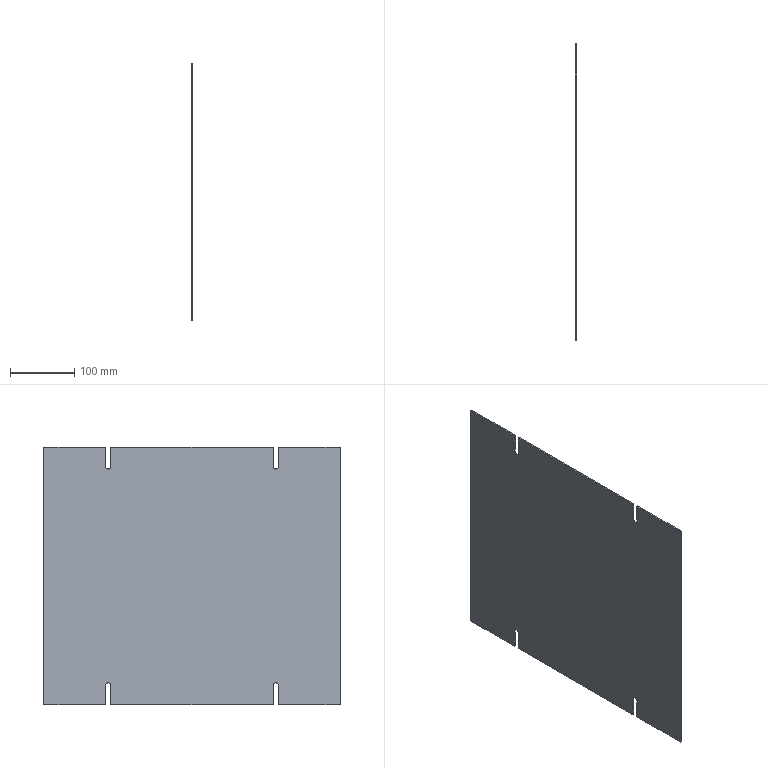Part | STEP file | Pneumatic circuit board | 1 solid | 24 faces | box 2 x 460 x 400 mm | volume 365879 mm3 | plane 18 | cylinder 6 | commonest cylinder face diameters 8 x6
STEP:
#1=CARTESIAN_POINT('',(0.,130.,166.));
#2=VERTEX_POINT('',#1);
#3=CARTESIAN_POINT('',(0.,134.,170.));
#4=VERTEX_POINT('',#3);
#5=CARTESIAN_POINT('',(0.,130.,170.));
#6=DIRECTION('',(1.,0.,0.));
#7=DIRECTION('',(0.,0.,-1.));
#8=AXIS2_PLACEMENT_3D('',#5,#6,#7);
#9=CIRCLE('',#8,4.);
#10=EDGE_CURVE('',#2,#4,#9,.T.);
#11=ORIENTED_EDGE('',*,*,#10,.F.);
#12=CARTESIAN_POINT('',(2.,130.,166.));
#13=VERTEX_POINT('',#12);
#14=CARTESIAN_POINT('',(0.,130.,166.));
#15=DIRECTION('',(1.,0.,0.));
#16=VECTOR('',#15,1000.);
#17=LINE('',#14,#16);
#18=EDGE_CURVE('',#2,#13,#17,.T.);
#19=ORIENTED_EDGE('',*,*,#18,.T.);
#20=CARTESIAN_POINT('',(2.,134.,170.));
#21=VERTEX_POINT('',#20);
#22=CARTESIAN_POINT('',(2.,130.,170.));
#23=DIRECTION('',(1.,0.,0.));
#24=DIRECTION('',(0.,0.,-1.));
#25=AXIS2_PLACEMENT_3D('',#22,#23,#24);
#26=CIRCLE('',#25,4.);
#27=EDGE_CURVE('',#13,#21,#26,.T.);
#28=ORIENTED_EDGE('',*,*,#27,.T.);
#29=CARTESIAN_POINT('',(0.,134.,170.));
#30=DIRECTION('',(-1.,0.,0.));
#31=VECTOR('',#30,1000.);
#32=LINE('',#29,#31);
#33=EDGE_CURVE('',#21,#4,#32,.T.);
#34=ORIENTED_EDGE('',*,*,#33,.T.);
#35=EDGE_LOOP('',(#11,#19,#28,#34));
#36=FACE_OUTER_BOUND('',#35,.T.);
#37=CARTESIAN_POINT('',(0.,130.,170.));
#38=DIRECTION('',(1.,0.,0.));
#39=DIRECTION('',(0.,0.,-1.));
#40=AXIS2_PLACEMENT_3D('',#37,#38,#39);
#41=CYLINDRICAL_SURFACE('',#40,4.);
#42=ADVANCED_FACE('',(#36),#41,.F.);
#43=CARTESIAN_POINT('',(0.,-130.,166.));
#44=VERTEX_POINT('',#43);
#45=CARTESIAN_POINT('',(0.,-126.,170.));
#46=VERTEX_POINT('',#45);
#47=CARTESIAN_POINT('',(0.,-130.,170.));
#48=DIRECTION('',(1.,0.,0.));
#49=DIRECTION('',(0.,0.,-1.));
#50=AXIS2_PLACEMENT_3D('',#47,#48,#49);
#51=CIRCLE('',#50,4.);
#52=EDGE_CURVE('',#44,#46,#51,.T.);
#53=ORIENTED_EDGE('',*,*,#52,.F.);
#54=CARTESIAN_POINT('',(2.,-130.,166.));
#55=VERTEX_POINT('',#54);
#56=CARTESIAN_POINT('',(0.,-130.,166.));
#57=DIRECTION('',(1.,0.,0.));
#58=VECTOR('',#57,1000.);
#59=LINE('',#56,#58);
#60=EDGE_CURVE('',#44,#55,#59,.T.);
#61=ORIENTED_EDGE('',*,*,#60,.T.);
#62=CARTESIAN_POINT('',(2.,-126.,170.));
#63=VERTEX_POINT('',#62);
#64=CARTESIAN_POINT('',(2.,-130.,170.));
#65=DIRECTION('',(1.,0.,0.));
#66=DIRECTION('',(0.,0.,-1.));
#67=AXIS2_PLACEMENT_3D('',#64,#65,#66);
#68=CIRCLE('',#67,4.);
#69=EDGE_CURVE('',#55,#63,#68,.T.);
#70=ORIENTED_EDGE('',*,*,#69,.T.);
#71=CARTESIAN_POINT('',(0.,-126.,170.));
#72=DIRECTION('',(-1.,0.,0.));
#73=VECTOR('',#72,1000.);
#74=LINE('',#71,#73);
#75=EDGE_CURVE('',#63,#46,#74,.T.);
#76=ORIENTED_EDGE('',*,*,#75,.T.);
#77=EDGE_LOOP('',(#53,#61,#70,#76));
#78=FACE_OUTER_BOUND('',#77,.T.);
#79=CARTESIAN_POINT('',(0.,-130.,170.));
#80=DIRECTION('',(1.,0.,0.));
#81=DIRECTION('',(0.,0.,-1.));
#82=AXIS2_PLACEMENT_3D('',#79,#80,#81);
#83=CYLINDRICAL_SURFACE('',#82,4.);
#84=ADVANCED_FACE('',(#78),#83,.F.);
#85=CARTESIAN_POINT('',(2.,134.,-170.));
#86=VERTEX_POINT('',#85);
#87=CARTESIAN_POINT('',(2.,126.,-170.));
#88=VERTEX_POINT('',#87);
#89=CARTESIAN_POINT('',(2.,130.,-170.));
#90=DIRECTION('',(1.,0.,0.));
#91=DIRECTION('',(0.,0.,-1.));
#92=AXIS2_PLACEMENT_3D('',#89,#90,#91);
#93=CIRCLE('',#92,4.);
#94=EDGE_CURVE('',#86,#88,#93,.T.);
#95=ORIENTED_EDGE('',*,*,#94,.F.);
#96=CARTESIAN_POINT('',(2.,134.,-200.));
#97=VERTEX_POINT('',#96);
#98=CARTESIAN_POINT('',(2.,134.,0.));
#99=DIRECTION('',(0.,0.,1.));
#100=VECTOR('',#99,1000.);
#101=LINE('',#98,#100);
#102=EDGE_CURVE('',#97,#86,#101,.T.);
#103=ORIENTED_EDGE('',*,*,#102,.F.);
#104=CARTESIAN_POINT('',(2.,230.,-200.));
#105=VERTEX_POINT('',#104);
#106=CARTESIAN_POINT('',(2.,0.,-200.));
#107=DIRECTION('',(0.,-1.,0.));
#108=VECTOR('',#107,1000.);
#109=LINE('',#106,#108);
#110=EDGE_CURVE('',#105,#97,#109,.T.);
#111=ORIENTED_EDGE('',*,*,#110,.F.);
#112=CARTESIAN_POINT('',(2.,230.,200.));
#113=VERTEX_POINT('',#112);
#114=CARTESIAN_POINT('',(2.,230.,0.));
#115=DIRECTION('',(0.,0.,-1.));
#116=VECTOR('',#115,1000.);
#117=LINE('',#114,#116);
#118=EDGE_CURVE('',#113,#105,#117,.T.);
#119=ORIENTED_EDGE('',*,*,#118,.F.);
#120=CARTESIAN_POINT('',(2.,134.,200.));
#121=VERTEX_POINT('',#120);
#122=CARTESIAN_POINT('',(2.,0.,200.));
#123=DIRECTION('',(0.,1.,0.));
#124=VECTOR('',#123,1000.);
#125=LINE('',#122,#124);
#126=EDGE_CURVE('',#121,#113,#125,.T.);
#127=ORIENTED_EDGE('',*,*,#126,.F.);
#128=CARTESIAN_POINT('',(2.,134.,0.));
#129=DIRECTION('',(0.,0.,1.));
#130=VECTOR('',#129,1000.);
#131=LINE('',#128,#130);
#132=EDGE_CURVE('',#21,#121,#131,.T.);
#133=ORIENTED_EDGE('',*,*,#132,.F.);
#134=ORIENTED_EDGE('',*,*,#27,.F.);
#135=CARTESIAN_POINT('',(2.,126.,170.));
#136=VERTEX_POINT('',#135);
#137=CARTESIAN_POINT('',(2.,130.,170.));
#138=DIRECTION('',(1.,0.,0.));
#139=DIRECTION('',(0.,0.,-1.));
#140=AXIS2_PLACEMENT_3D('',#137,#138,#139);
#141=CIRCLE('',#140,4.);
#142=EDGE_CURVE('',#136,#13,#141,.T.);
#143=ORIENTED_EDGE('',*,*,#142,.F.);
#144=CARTESIAN_POINT('',(2.,126.,200.));
#145=VERTEX_POINT('',#144);
#146=CARTESIAN_POINT('',(2.,126.,0.));
#147=DIRECTION('',(0.,0.,-1.));
#148=VECTOR('',#147,1000.);
#149=LINE('',#146,#148);
#150=EDGE_CURVE('',#145,#136,#149,.T.);
#151=ORIENTED_EDGE('',*,*,#150,.F.);
#152=CARTESIAN_POINT('',(2.,-126.,200.));
#153=VERTEX_POINT('',#152);
#154=CARTESIAN_POINT('',(2.,0.,200.));
#155=DIRECTION('',(0.,1.,0.));
#156=VECTOR('',#155,1000.);
#157=LINE('',#154,#156);
#158=EDGE_CURVE('',#153,#145,#157,.T.);
#159=ORIENTED_EDGE('',*,*,#158,.F.);
#160=CARTESIAN_POINT('',(2.,-126.,0.));
#161=DIRECTION('',(0.,0.,1.));
#162=VECTOR('',#161,1000.);
#163=LINE('',#160,#162);
#164=EDGE_CURVE('',#63,#153,#163,.T.);
#165=ORIENTED_EDGE('',*,*,#164,.F.);
#166=ORIENTED_EDGE('',*,*,#69,.F.);
#167=CARTESIAN_POINT('',(2.,-134.,170.));
#168=VERTEX_POINT('',#167);
#169=CARTESIAN_POINT('',(2.,-130.,170.));
#170=DIRECTION('',(1.,0.,0.));
#171=DIRECTION('',(0.,0.,-1.));
#172=AXIS2_PLACEMENT_3D('',#169,#170,#171);
#173=CIRCLE('',#172,4.);
#174=EDGE_CURVE('',#168,#55,#173,.T.);
#175=ORIENTED_EDGE('',*,*,#174,.F.);
#176=CARTESIAN_POINT('',(2.,-134.,200.));
#177=VERTEX_POINT('',#176);
#178=CARTESIAN_POINT('',(2.,-134.,0.));
#179=DIRECTION('',(0.,0.,-1.));
#180=VECTOR('',#179,1000.);
#181=LINE('',#178,#180);
#182=EDGE_CURVE('',#177,#168,#181,.T.);
#183=ORIENTED_EDGE('',*,*,#182,.F.);
#184=CARTESIAN_POINT('',(2.,-230.,200.));
#185=VERTEX_POINT('',#184);
#186=CARTESIAN_POINT('',(2.,0.,200.));
#187=DIRECTION('',(0.,1.,0.));
#188=VECTOR('',#187,1000.);
#189=LINE('',#186,#188);
#190=EDGE_CURVE('',#185,#177,#189,.T.);
#191=ORIENTED_EDGE('',*,*,#190,.F.);
#192=CARTESIAN_POINT('',(2.,-230.,-200.));
#193=VERTEX_POINT('',#192);
#194=CARTESIAN_POINT('',(2.,-230.,0.));
#195=DIRECTION('',(0.,0.,1.));
#196=VECTOR('',#195,1000.);
#197=LINE('',#194,#196);
#198=EDGE_CURVE('',#193,#185,#197,.T.);
#199=ORIENTED_EDGE('',*,*,#198,.F.);
#200=CARTESIAN_POINT('',(2.,-134.,-200.));
#201=VERTEX_POINT('',#200);
#202=CARTESIAN_POINT('',(2.,0.,-200.));
#203=DIRECTION('',(0.,-1.,0.));
#204=VECTOR('',#203,1000.);
#205=LINE('',#202,#204);
#206=EDGE_CURVE('',#201,#193,#205,.T.);
#207=ORIENTED_EDGE('',*,*,#206,.F.);
#208=CARTESIAN_POINT('',(2.,-134.,-170.));
#209=VERTEX_POINT('',#208);
#210=CARTESIAN_POINT('',(2.,-134.,0.));
#211=DIRECTION('',(0.,0.,-1.));
#212=VECTOR('',#211,1000.);
#213=LINE('',#210,#212);
#214=EDGE_CURVE('',#209,#201,#213,.T.);
#215=ORIENTED_EDGE('',*,*,#214,.F.);
#216=CARTESIAN_POINT('',(2.,-126.,-170.));
#217=VERTEX_POINT('',#216);
#218=CARTESIAN_POINT('',(2.,-130.,-170.));
#219=DIRECTION('',(1.,0.,0.));
#220=DIRECTION('',(0.,0.,-1.));
#221=AXIS2_PLACEMENT_3D('',#218,#219,#220);
#222=CIRCLE('',#221,4.);
#223=EDGE_CURVE('',#217,#209,#222,.T.);
#224=ORIENTED_EDGE('',*,*,#223,.F.);
#225=CARTESIAN_POINT('',(2.,-126.,-200.));
#226=VERTEX_POINT('',#225);
#227=CARTESIAN_POINT('',(2.,-126.,0.));
#228=DIRECTION('',(0.,0.,1.));
#229=VECTOR('',#228,1000.);
#230=LINE('',#227,#229);
#231=EDGE_CURVE('',#226,#217,#230,.T.);
#232=ORIENTED_EDGE('',*,*,#231,.F.);
#233=CARTESIAN_POINT('',(2.,126.,-200.));
#234=VERTEX_POINT('',#233);
#235=CARTESIAN_POINT('',(2.,0.,-200.));
#236=DIRECTION('',(0.,-1.,0.));
#237=VECTOR('',#236,1000.);
#238=LINE('',#235,#237);
#239=EDGE_CURVE('',#234,#226,#238,.T.);
#240=ORIENTED_EDGE('',*,*,#239,.F.);
#241=CARTESIAN_POINT('',(2.,126.,0.));
#242=DIRECTION('',(0.,0.,-1.));
#243=VECTOR('',#242,1000.);
#244=LINE('',#241,#243);
#245=EDGE_CURVE('',#88,#234,#244,.T.);
#246=ORIENTED_EDGE('',*,*,#245,.F.);
#247=EDGE_LOOP('',(#95,#103,#111,#119,#127,#133,#134,#143,#151,#159,#165,#166,#175,#183,#191,#199,#207,#215,#224,#232,#240,#246));
#248=FACE_OUTER_BOUND('',#247,.T.);
#249=CARTESIAN_POINT('',(2.,0.,0.));
#250=DIRECTION('',(-1.,0.,0.));
#251=DIRECTION('',(0.,0.,1.));
#252=AXIS2_PLACEMENT_3D('',#249,#250,#251);
#253=PLANE('',#252);
#254=ADVANCED_FACE('',(#248),#253,.F.);
#255=CARTESIAN_POINT('',(0.,126.,-170.));
#256=VERTEX_POINT('',#255);
#257=CARTESIAN_POINT('',(0.,126.,-170.));
#258=DIRECTION('',(1.,0.,0.));
#259=VECTOR('',#258,1000.);
#260=LINE('',#257,#259);
#261=EDGE_CURVE('',#256,#88,#260,.T.);
#262=ORIENTED_EDGE('',*,*,#261,.T.);
#263=ORIENTED_EDGE('',*,*,#245,.T.);
#264=CARTESIAN_POINT('',(0.,126.,-200.));
#265=VERTEX_POINT('',#264);
#266=CARTESIAN_POINT('',(0.,126.,-200.));
#267=DIRECTION('',(-1.,0.,0.));
#268=VECTOR('',#267,1000.);
#269=LINE('',#266,#268);
#270=EDGE_CURVE('',#234,#265,#269,.T.);
#271=ORIENTED_EDGE('',*,*,#270,.T.);
#272=CARTESIAN_POINT('',(0.,126.,-230.));
#273=DIRECTION('',(0.,0.,1.));
#274=VECTOR('',#273,1000.);
#275=LINE('',#272,#274);
#276=EDGE_CURVE('',#265,#256,#275,.T.);
#277=ORIENTED_EDGE('',*,*,#276,.T.);
#278=EDGE_LOOP('',(#262,#263,#271,#277));
#279=FACE_OUTER_BOUND('',#278,.T.);
#280=CARTESIAN_POINT('',(0.,126.,-230.));
#281=DIRECTION('',(0.,1.,0.));
#282=DIRECTION('',(0.,0.,1.));
#283=AXIS2_PLACEMENT_3D('',#280,#281,#282);
#284=PLANE('',#283);
#285=ADVANCED_FACE('',(#279),#284,.T.);
#286=ORIENTED_EDGE('',*,*,#261,.F.);
#287=CARTESIAN_POINT('',(0.,134.,-170.));
#288=VERTEX_POINT('',#287);
#289=CARTESIAN_POINT('',(0.,130.,-170.));
#290=DIRECTION('',(1.,0.,0.));
#291=DIRECTION('',(0.,0.,-1.));
#292=AXIS2_PLACEMENT_3D('',#289,#290,#291);
#293=CIRCLE('',#292,4.);
#294=EDGE_CURVE('',#288,#256,#293,.T.);
#295=ORIENTED_EDGE('',*,*,#294,.F.);
#296=CARTESIAN_POINT('',(0.,134.,-170.));
#297=DIRECTION('',(-1.,0.,0.));
#298=VECTOR('',#297,1000.);
#299=LINE('',#296,#298);
#300=EDGE_CURVE('',#86,#288,#299,.T.);
#301=ORIENTED_EDGE('',*,*,#300,.F.);
#302=ORIENTED_EDGE('',*,*,#94,.T.);
#303=EDGE_LOOP('',(#286,#295,#301,#302));
#304=FACE_OUTER_BOUND('',#303,.T.);
#305=CARTESIAN_POINT('',(0.,130.,-170.));
#306=DIRECTION('',(1.,0.,0.));
#307=DIRECTION('',(0.,0.,-1.));
#308=AXIS2_PLACEMENT_3D('',#305,#306,#307);
#309=CYLINDRICAL_SURFACE('',#308,4.);
#310=ADVANCED_FACE('',(#304),#309,.F.);
#311=ORIENTED_EDGE('',*,*,#300,.T.);
#312=CARTESIAN_POINT('',(0.,134.,-200.));
#313=VERTEX_POINT('',#312);
#314=CARTESIAN_POINT('',(0.,134.,-230.));
#315=DIRECTION('',(0.,0.,-1.));
#316=VECTOR('',#315,1000.);
#317=LINE('',#314,#316);
#318=EDGE_CURVE('',#288,#313,#317,.T.);
#319=ORIENTED_EDGE('',*,*,#318,.T.);
#320=CARTESIAN_POINT('',(0.,134.,-200.));
#321=DIRECTION('',(1.,0.,0.));
#322=VECTOR('',#321,1000.);
#323=LINE('',#320,#322);
#324=EDGE_CURVE('',#313,#97,#323,.T.);
#325=ORIENTED_EDGE('',*,*,#324,.T.);
#326=ORIENTED_EDGE('',*,*,#102,.T.);
#327=EDGE_LOOP('',(#311,#319,#325,#326));
#328=FACE_OUTER_BOUND('',#327,.T.);
#329=CARTESIAN_POINT('',(0.,134.,-230.));
#330=DIRECTION('',(0.,-1.,0.));
#331=DIRECTION('',(0.,0.,-1.));
#332=AXIS2_PLACEMENT_3D('',#329,#330,#331);
#333=PLANE('',#332);
#334=ADVANCED_FACE('',(#328),#333,.T.);
#335=CARTESIAN_POINT('',(0.,230.,-200.));
#336=VERTEX_POINT('',#335);
#337=CARTESIAN_POINT('',(0.,-230.,-200.));
#338=DIRECTION('',(0.,-1.,0.));
#339=VECTOR('',#338,1000.);
#340=LINE('',#337,#339);
#341=EDGE_CURVE('',#336,#313,#340,.T.);
#342=ORIENTED_EDGE('',*,*,#341,.F.);
#343=CARTESIAN_POINT('',(2.,230.,-200.));
#344=DIRECTION('',(-1.,0.,0.));
#345=VECTOR('',#344,1000.);
#346=LINE('',#343,#345);
#347=EDGE_CURVE('',#105,#336,#346,.T.);
#348=ORIENTED_EDGE('',*,*,#347,.F.);
#349=ORIENTED_EDGE('',*,*,#110,.T.);
#350=ORIENTED_EDGE('',*,*,#324,.F.);
#351=EDGE_LOOP('',(#342,#348,#349,#350));
#352=FACE_OUTER_BOUND('',#351,.T.);
#353=CARTESIAN_POINT('',(2.,-230.,-200.));
#354=DIRECTION('',(0.,0.,1.));
#355=DIRECTION('',(1.,0.,0.));
#356=AXIS2_PLACEMENT_3D('',#353,#354,#355);
#357=PLANE('',#356);
#358=ADVANCED_FACE('',(#352),#357,.F.);
#359=CARTESIAN_POINT('',(0.,230.,200.));
#360=VERTEX_POINT('',#359);
#361=CARTESIAN_POINT('',(2.,230.,200.));
#362=DIRECTION('',(-1.,0.,0.));
#363=VECTOR('',#362,1000.);
#364=LINE('',#361,#363);
#365=EDGE_CURVE('',#113,#360,#364,.T.);
#366=ORIENTED_EDGE('',*,*,#365,.F.);
#367=ORIENTED_EDGE('',*,*,#118,.T.);
#368=ORIENTED_EDGE('',*,*,#347,.T.);
#369=CARTESIAN_POINT('',(0.,230.,200.));
#370=DIRECTION('',(0.,0.,-1.));
#371=VECTOR('',#370,1000.);
#372=LINE('',#369,#371);
#373=EDGE_CURVE('',#360,#336,#372,.T.);
#374=ORIENTED_EDGE('',*,*,#373,.F.);
#375=EDGE_LOOP('',(#366,#367,#368,#374));
#376=FACE_OUTER_BOUND('',#375,.T.);
#377=CARTESIAN_POINT('',(2.,230.,200.));
#378=DIRECTION('',(0.,-1.,0.));
#379=DIRECTION('',(0.,0.,-1.));
#380=AXIS2_PLACEMENT_3D('',#377,#378,#379);
#381=PLANE('',#380);
#382=ADVANCED_FACE('',(#376),#381,.F.);
#383=CARTESIAN_POINT('',(0.,134.,200.));
#384=VERTEX_POINT('',#383);
#385=CARTESIAN_POINT('',(2.,134.,200.));
#386=DIRECTION('',(-1.,0.,0.));
#387=VECTOR('',#386,1000.);
#388=LINE('',#385,#387);
#389=EDGE_CURVE('',#121,#384,#388,.T.);
#390=ORIENTED_EDGE('',*,*,#389,.F.);
#391=ORIENTED_EDGE('',*,*,#126,.T.);
#392=ORIENTED_EDGE('',*,*,#365,.T.);
#393=CARTESIAN_POINT('',(0.,-230.,200.));
#394=DIRECTION('',(0.,1.,0.));
#395=VECTOR('',#394,1000.);
#396=LINE('',#393,#395);
#397=EDGE_CURVE('',#384,#360,#396,.T.);
#398=ORIENTED_EDGE('',*,*,#397,.F.);
#399=EDGE_LOOP('',(#390,#391,#392,#398));
#400=FACE_OUTER_BOUND('',#399,.T.);
#401=CARTESIAN_POINT('',(2.,-230.,200.));
#402=DIRECTION('',(0.,0.,-1.));
#403=DIRECTION('',(-1.,0.,0.));
#404=AXIS2_PLACEMENT_3D('',#401,#402,#403);
#405=PLANE('',#404);
#406=ADVANCED_FACE('',(#400),#405,.F.);
#407=ORIENTED_EDGE('',*,*,#33,.F.);
#408=ORIENTED_EDGE('',*,*,#132,.T.);
#409=ORIENTED_EDGE('',*,*,#389,.T.);
#410=CARTESIAN_POINT('',(0.,134.,230.));
#411=DIRECTION('',(0.,0.,1.));
#412=VECTOR('',#411,1000.);
#413=LINE('',#410,#412);
#414=EDGE_CURVE('',#4,#384,#413,.T.);
#415=ORIENTED_EDGE('',*,*,#414,.F.);
#416=EDGE_LOOP('',(#407,#408,#409,#415));
#417=FACE_OUTER_BOUND('',#416,.T.);
#418=CARTESIAN_POINT('',(0.,134.,230.));
#419=DIRECTION('',(0.,1.,0.));
#420=DIRECTION('',(0.,0.,1.));
#421=AXIS2_PLACEMENT_3D('',#418,#419,#420);
#422=PLANE('',#421);
#423=ADVANCED_FACE('',(#417),#422,.F.);
#424=ORIENTED_EDGE('',*,*,#18,.F.);
#425=CARTESIAN_POINT('',(0.,126.,170.));
#426=VERTEX_POINT('',#425);
#427=CARTESIAN_POINT('',(0.,130.,170.));
#428=DIRECTION('',(1.,0.,0.));
#429=DIRECTION('',(0.,0.,-1.));
#430=AXIS2_PLACEMENT_3D('',#427,#428,#429);
#431=CIRCLE('',#430,4.);
#432=EDGE_CURVE('',#426,#2,#431,.T.);
#433=ORIENTED_EDGE('',*,*,#432,.F.);
#434=CARTESIAN_POINT('',(0.,126.,170.));
#435=DIRECTION('',(-1.,0.,0.));
#436=VECTOR('',#435,1000.);
#437=LINE('',#434,#436);
#438=EDGE_CURVE('',#136,#426,#437,.T.);
#439=ORIENTED_EDGE('',*,*,#438,.F.);
#440=ORIENTED_EDGE('',*,*,#142,.T.);
#441=EDGE_LOOP('',(#424,#433,#439,#440));
#442=FACE_OUTER_BOUND('',#441,.T.);
#443=CARTESIAN_POINT('',(0.,130.,170.));
#444=DIRECTION('',(1.,0.,0.));
#445=DIRECTION('',(0.,0.,-1.));
#446=AXIS2_PLACEMENT_3D('',#443,#444,#445);
#447=CYLINDRICAL_SURFACE('',#446,4.);
#448=ADVANCED_FACE('',(#442),#447,.F.);
#449=ORIENTED_EDGE('',*,*,#438,.T.);
#450=CARTESIAN_POINT('',(0.,126.,200.));
#451=VERTEX_POINT('',#450);
#452=CARTESIAN_POINT('',(0.,126.,230.));
#453=DIRECTION('',(0.,0.,-1.));
#454=VECTOR('',#453,1000.);
#455=LINE('',#452,#454);
#456=EDGE_CURVE('',#451,#426,#455,.T.);
#457=ORIENTED_EDGE('',*,*,#456,.F.);
#458=CARTESIAN_POINT('',(0.,126.,200.));
#459=DIRECTION('',(-1.,0.,0.));
#460=VECTOR('',#459,1000.);
#461=LINE('',#458,#460);
#462=EDGE_CURVE('',#145,#451,#461,.T.);
#463=ORIENTED_EDGE('',*,*,#462,.F.);
#464=ORIENTED_EDGE('',*,*,#150,.T.);
#465=EDGE_LOOP('',(#449,#457,#463,#464));
#466=FACE_OUTER_BOUND('',#465,.T.);
#467=CARTESIAN_POINT('',(0.,126.,230.));
#468=DIRECTION('',(0.,-1.,0.));
#469=DIRECTION('',(0.,0.,-1.));
#470=AXIS2_PLACEMENT_3D('',#467,#468,#469);
#471=PLANE('',#470);
#472=ADVANCED_FACE('',(#466),#471,.F.);
#473=ORIENTED_EDGE('',*,*,#462,.T.);
#474=CARTESIAN_POINT('',(0.,-126.,200.));
#475=VERTEX_POINT('',#474);
#476=CARTESIAN_POINT('',(0.,-230.,200.));
#477=DIRECTION('',(0.,1.,0.));
#478=VECTOR('',#477,1000.);
#479=LINE('',#476,#478);
#480=EDGE_CURVE('',#475,#451,#479,.T.);
#481=ORIENTED_EDGE('',*,*,#480,.F.);
#482=CARTESIAN_POINT('',(2.,-126.,200.));
#483=DIRECTION('',(-1.,0.,0.));
#484=VECTOR('',#483,1000.);
#485=LINE('',#482,#484);
#486=EDGE_CURVE('',#153,#475,#485,.T.);
#487=ORIENTED_EDGE('',*,*,#486,.F.);
#488=ORIENTED_EDGE('',*,*,#158,.T.);
#489=EDGE_LOOP('',(#473,#481,#487,#488));
#490=FACE_OUTER_BOUND('',#489,.T.);
#491=CARTESIAN_POINT('',(2.,-230.,200.));
#492=DIRECTION('',(0.,0.,-1.));
#493=DIRECTION('',(-1.,0.,0.));
#494=AXIS2_PLACEMENT_3D('',#491,#492,#493);
#495=PLANE('',#494);
#496=ADVANCED_FACE('',(#490),#495,.F.);
#497=ORIENTED_EDGE('',*,*,#75,.F.);
#498=ORIENTED_EDGE('',*,*,#164,.T.);
#499=ORIENTED_EDGE('',*,*,#486,.T.);
#500=CARTESIAN_POINT('',(0.,-126.,230.));
#501=DIRECTION('',(0.,0.,1.));
#502=VECTOR('',#501,1000.);
#503=LINE('',#500,#502);
#504=EDGE_CURVE('',#46,#475,#503,.T.);
#505=ORIENTED_EDGE('',*,*,#504,.F.);
#506=EDGE_LOOP('',(#497,#498,#499,#505));
#507=FACE_OUTER_BOUND('',#506,.T.);
#508=CARTESIAN_POINT('',(0.,-126.,230.));
#509=DIRECTION('',(0.,1.,0.));
#510=DIRECTION('',(0.,0.,1.));
#511=AXIS2_PLACEMENT_3D('',#508,#509,#510);
#512=PLANE('',#511);
#513=ADVANCED_FACE('',(#507),#512,.F.);
#514=ORIENTED_EDGE('',*,*,#60,.F.);
#515=CARTESIAN_POINT('',(0.,-134.,170.));
#516=VERTEX_POINT('',#515);
#517=CARTESIAN_POINT('',(0.,-130.,170.));
#518=DIRECTION('',(1.,0.,0.));
#519=DIRECTION('',(0.,0.,-1.));
#520=AXIS2_PLACEMENT_3D('',#517,#518,#519);
#521=CIRCLE('',#520,4.);
#522=EDGE_CURVE('',#516,#44,#521,.T.);
#523=ORIENTED_EDGE('',*,*,#522,.F.);
#524=CARTESIAN_POINT('',(0.,-134.,170.));
#525=DIRECTION('',(-1.,0.,0.));
#526=VECTOR('',#525,1000.);
#527=LINE('',#524,#526);
#528=EDGE_CURVE('',#168,#516,#527,.T.);
#529=ORIENTED_EDGE('',*,*,#528,.F.);
#530=ORIENTED_EDGE('',*,*,#174,.T.);
#531=EDGE_LOOP('',(#514,#523,#529,#530));
#532=FACE_OUTER_BOUND('',#531,.T.);
#533=CARTESIAN_POINT('',(0.,-130.,170.));
#534=DIRECTION('',(1.,0.,0.));
#535=DIRECTION('',(0.,0.,-1.));
#536=AXIS2_PLACEMENT_3D('',#533,#534,#535);
#537=CYLINDRICAL_SURFACE('',#536,4.);
#538=ADVANCED_FACE('',(#532),#537,.F.);
#539=ORIENTED_EDGE('',*,*,#528,.T.);
#540=CARTESIAN_POINT('',(0.,-134.,200.));
#541=VERTEX_POINT('',#540);
#542=CARTESIAN_POINT('',(0.,-134.,230.));
#543=DIRECTION('',(0.,0.,-1.));
#544=VECTOR('',#543,1000.);
#545=LINE('',#542,#544);
#546=EDGE_CURVE('',#541,#516,#545,.T.);
#547=ORIENTED_EDGE('',*,*,#546,.F.);
#548=CARTESIAN_POINT('',(0.,-134.,200.));
#549=DIRECTION('',(-1.,0.,0.));
#550=VECTOR('',#549,1000.);
#551=LINE('',#548,#550);
#552=EDGE_CURVE('',#177,#541,#551,.T.);
#553=ORIENTED_EDGE('',*,*,#552,.F.);
#554=ORIENTED_EDGE('',*,*,#182,.T.);
#555=EDGE_LOOP('',(#539,#547,#553,#554));
#556=FACE_OUTER_BOUND('',#555,.T.);
#557=CARTESIAN_POINT('',(0.,-134.,230.));
#558=DIRECTION('',(0.,-1.,0.));
#559=DIRECTION('',(0.,0.,-1.));
#560=AXIS2_PLACEMENT_3D('',#557,#558,#559);
#561=PLANE('',#560);
#562=ADVANCED_FACE('',(#556),#561,.F.);
#563=ORIENTED_EDGE('',*,*,#552,.T.);
#564=CARTESIAN_POINT('',(0.,-230.,200.));
#565=VERTEX_POINT('',#564);
#566=CARTESIAN_POINT('',(0.,-230.,200.));
#567=DIRECTION('',(0.,1.,0.));
#568=VECTOR('',#567,1000.);
#569=LINE('',#566,#568);
#570=EDGE_CURVE('',#565,#541,#569,.T.);
#571=ORIENTED_EDGE('',*,*,#570,.F.);
#572=CARTESIAN_POINT('',(2.,-230.,200.));
#573=DIRECTION('',(-1.,0.,0.));
#574=VECTOR('',#573,1000.);
#575=LINE('',#572,#574);
#576=EDGE_CURVE('',#185,#565,#575,.T.);
#577=ORIENTED_EDGE('',*,*,#576,.F.);
#578=ORIENTED_EDGE('',*,*,#190,.T.);
#579=EDGE_LOOP('',(#563,#571,#577,#578));
#580=FACE_OUTER_BOUND('',#579,.T.);
#581=CARTESIAN_POINT('',(2.,-230.,200.));
#582=DIRECTION('',(0.,0.,-1.));
#583=DIRECTION('',(-1.,0.,0.));
#584=AXIS2_PLACEMENT_3D('',#581,#582,#583);
#585=PLANE('',#584);
#586=ADVANCED_FACE('',(#580),#585,.F.);
#587=CARTESIAN_POINT('',(0.,-230.,-200.));
#588=VERTEX_POINT('',#587);
#589=CARTESIAN_POINT('',(2.,-230.,-200.));
#590=DIRECTION('',(-1.,0.,0.));
#591=VECTOR('',#590,1000.);
#592=LINE('',#589,#591);
#593=EDGE_CURVE('',#193,#588,#592,.T.);
#594=ORIENTED_EDGE('',*,*,#593,.F.);
#595=ORIENTED_EDGE('',*,*,#198,.T.);
#596=ORIENTED_EDGE('',*,*,#576,.T.);
#597=CARTESIAN_POINT('',(0.,-230.,200.));
#598=DIRECTION('',(0.,0.,1.));
#599=VECTOR('',#598,1000.);
#600=LINE('',#597,#599);
#601=EDGE_CURVE('',#588,#565,#600,.T.);
#602=ORIENTED_EDGE('',*,*,#601,.F.);
#603=EDGE_LOOP('',(#594,#595,#596,#602));
#604=FACE_OUTER_BOUND('',#603,.T.);
#605=CARTESIAN_POINT('',(2.,-230.,200.));
#606=DIRECTION('',(0.,1.,0.));
#607=DIRECTION('',(0.,0.,1.));
#608=AXIS2_PLACEMENT_3D('',#605,#606,#607);
#609=PLANE('',#608);
#610=ADVANCED_FACE('',(#604),#609,.F.);
#611=ORIENTED_EDGE('',*,*,#206,.T.);
#612=ORIENTED_EDGE('',*,*,#593,.T.);
#613=CARTESIAN_POINT('',(0.,-134.,-200.));
#614=VERTEX_POINT('',#613);
#615=CARTESIAN_POINT('',(0.,-230.,-200.));
#616=DIRECTION('',(0.,-1.,0.));
#617=VECTOR('',#616,1000.);
#618=LINE('',#615,#617);
#619=EDGE_CURVE('',#614,#588,#618,.T.);
#620=ORIENTED_EDGE('',*,*,#619,.F.);
#621=CARTESIAN_POINT('',(2.,-134.,-200.));
#622=DIRECTION('',(-1.,0.,0.));
#623=VECTOR('',#622,1000.);
#624=LINE('',#621,#623);
#625=EDGE_CURVE('',#201,#614,#624,.T.);
#626=ORIENTED_EDGE('',*,*,#625,.F.);
#627=EDGE_LOOP('',(#611,#612,#620,#626));
#628=FACE_OUTER_BOUND('',#627,.T.);
#629=CARTESIAN_POINT('',(2.,-230.,-200.));
#630=DIRECTION('',(0.,0.,1.));
#631=DIRECTION('',(1.,0.,0.));
#632=AXIS2_PLACEMENT_3D('',#629,#630,#631);
#633=PLANE('',#632);
#634=ADVANCED_FACE('',(#628),#633,.F.);
#635=CARTESIAN_POINT('',(0.,-134.,-170.));
#636=VERTEX_POINT('',#635);
#637=CARTESIAN_POINT('',(0.,-134.,-170.));
#638=DIRECTION('',(1.,0.,0.));
#639=VECTOR('',#638,1000.);
#640=LINE('',#637,#639);
#641=EDGE_CURVE('',#636,#209,#640,.T.);
#642=ORIENTED_EDGE('',*,*,#641,.T.);
#643=ORIENTED_EDGE('',*,*,#214,.T.);
#644=ORIENTED_EDGE('',*,*,#625,.T.);
#645=CARTESIAN_POINT('',(0.,-134.,-230.));
#646=DIRECTION('',(0.,0.,1.));
#647=VECTOR('',#646,1000.);
#648=LINE('',#645,#647);
#649=EDGE_CURVE('',#614,#636,#648,.T.);
#650=ORIENTED_EDGE('',*,*,#649,.T.);
#651=EDGE_LOOP('',(#642,#643,#644,#650));
#652=FACE_OUTER_BOUND('',#651,.T.);
#653=CARTESIAN_POINT('',(0.,-134.,-230.));
#654=DIRECTION('',(0.,1.,0.));
#655=DIRECTION('',(0.,0.,1.));
#656=AXIS2_PLACEMENT_3D('',#653,#654,#655);
#657=PLANE('',#656);
#658=ADVANCED_FACE('',(#652),#657,.T.);
#659=ORIENTED_EDGE('',*,*,#641,.F.);
#660=CARTESIAN_POINT('',(0.,-126.,-170.));
#661=VERTEX_POINT('',#660);
#662=CARTESIAN_POINT('',(0.,-130.,-170.));
#663=DIRECTION('',(1.,0.,0.));
#664=DIRECTION('',(0.,0.,-1.));
#665=AXIS2_PLACEMENT_3D('',#662,#663,#664);
#666=CIRCLE('',#665,4.);
#667=EDGE_CURVE('',#661,#636,#666,.T.);
#668=ORIENTED_EDGE('',*,*,#667,.F.);
#669=CARTESIAN_POINT('',(0.,-126.,-170.));
#670=DIRECTION('',(-1.,0.,0.));
#671=VECTOR('',#670,1000.);
#672=LINE('',#669,#671);
#673=EDGE_CURVE('',#217,#661,#672,.T.);
#674=ORIENTED_EDGE('',*,*,#673,.F.);
#675=ORIENTED_EDGE('',*,*,#223,.T.);
#676=EDGE_LOOP('',(#659,#668,#674,#675));
#677=FACE_OUTER_BOUND('',#676,.T.);
#678=CARTESIAN_POINT('',(0.,-130.,-170.));
#679=DIRECTION('',(1.,0.,0.));
#680=DIRECTION('',(0.,0.,-1.));
#681=AXIS2_PLACEMENT_3D('',#678,#679,#680);
#682=CYLINDRICAL_SURFACE('',#681,4.);
#683=ADVANCED_FACE('',(#677),#682,.F.);
#684=ORIENTED_EDGE('',*,*,#673,.T.);
#685=CARTESIAN_POINT('',(0.,-126.,-200.));
#686=VERTEX_POINT('',#685);
#687=CARTESIAN_POINT('',(0.,-126.,-230.));
#688=DIRECTION('',(0.,0.,-1.));
#689=VECTOR('',#688,1000.);
#690=LINE('',#687,#689);
#691=EDGE_CURVE('',#661,#686,#690,.T.);
#692=ORIENTED_EDGE('',*,*,#691,.T.);
#693=CARTESIAN_POINT('',(0.,-126.,-200.));
#694=DIRECTION('',(1.,0.,0.));
#695=VECTOR('',#694,1000.);
#696=LINE('',#693,#695);
#697=EDGE_CURVE('',#686,#226,#696,.T.);
#698=ORIENTED_EDGE('',*,*,#697,.T.);
#699=ORIENTED_EDGE('',*,*,#231,.T.);
#700=EDGE_LOOP('',(#684,#692,#698,#699));
#701=FACE_OUTER_BOUND('',#700,.T.);
#702=CARTESIAN_POINT('',(0.,-126.,-230.));
#703=DIRECTION('',(0.,-1.,0.));
#704=DIRECTION('',(0.,0.,-1.));
#705=AXIS2_PLACEMENT_3D('',#702,#703,#704);
#706=PLANE('',#705);
#707=ADVANCED_FACE('',(#701),#706,.T.);
#708=ORIENTED_EDGE('',*,*,#239,.T.);
#709=ORIENTED_EDGE('',*,*,#697,.F.);
#710=CARTESIAN_POINT('',(0.,-230.,-200.));
#711=DIRECTION('',(0.,-1.,0.));
#712=VECTOR('',#711,1000.);
#713=LINE('',#710,#712);
#714=EDGE_CURVE('',#265,#686,#713,.T.);
#715=ORIENTED_EDGE('',*,*,#714,.F.);
#716=ORIENTED_EDGE('',*,*,#270,.F.);
#717=EDGE_LOOP('',(#708,#709,#715,#716));
#718=FACE_OUTER_BOUND('',#717,.T.);
#719=CARTESIAN_POINT('',(2.,-230.,-200.));
#720=DIRECTION('',(0.,0.,1.));
#721=DIRECTION('',(1.,0.,0.));
#722=AXIS2_PLACEMENT_3D('',#719,#720,#721);
#723=PLANE('',#722);
#724=ADVANCED_FACE('',(#718),#723,.F.);
#725=ORIENTED_EDGE('',*,*,#341,.T.);
#726=ORIENTED_EDGE('',*,*,#318,.F.);
#727=ORIENTED_EDGE('',*,*,#294,.T.);
#728=ORIENTED_EDGE('',*,*,#276,.F.);
#729=ORIENTED_EDGE('',*,*,#714,.T.);
#730=ORIENTED_EDGE('',*,*,#691,.F.);
#731=ORIENTED_EDGE('',*,*,#667,.T.);
#732=ORIENTED_EDGE('',*,*,#649,.F.);
#733=ORIENTED_EDGE('',*,*,#619,.T.);
#734=ORIENTED_EDGE('',*,*,#601,.T.);
#735=ORIENTED_EDGE('',*,*,#570,.T.);
#736=ORIENTED_EDGE('',*,*,#546,.T.);
#737=ORIENTED_EDGE('',*,*,#522,.T.);
#738=ORIENTED_EDGE('',*,*,#52,.T.);
#739=ORIENTED_EDGE('',*,*,#504,.T.);
#740=ORIENTED_EDGE('',*,*,#480,.T.);
#741=ORIENTED_EDGE('',*,*,#456,.T.);
#742=ORIENTED_EDGE('',*,*,#432,.T.);
#743=ORIENTED_EDGE('',*,*,#10,.T.);
#744=ORIENTED_EDGE('',*,*,#414,.T.);
#745=ORIENTED_EDGE('',*,*,#397,.T.);
#746=ORIENTED_EDGE('',*,*,#373,.T.);
#747=EDGE_LOOP('',(#725,#726,#727,#728,#729,#730,#731,#732,#733,#734,#735,#736,#737,#738,#739,#740,#741,#742,#743,#744,#745,#746));
#748=FACE_OUTER_BOUND('',#747,.T.);
#749=CARTESIAN_POINT('',(0.,0.,0.));
#750=DIRECTION('',(-1.,0.,0.));
#751=DIRECTION('',(0.,0.,1.));
#752=AXIS2_PLACEMENT_3D('',#749,#750,#751);
#753=PLANE('',#752);
#754=ADVANCED_FACE('',(#748),#753,.T.);
#755=CLOSED_SHELL('',(#42,#84,#254,#285,#310,#334,#358,#382,#406,#423,#448,#472,#496,#513,#538,#562,#586,#610,#634,#658,#683,#707,#724,#754));
#756=MANIFOLD_SOLID_BREP('',#755);
#757=CARTESIAN_POINT('',(0.,0.,0.));
#758=DIRECTION('',(0.,0.,1.));
#759=DIRECTION('',(1.,0.,0.));
#760=AXIS2_PLACEMENT_3D('',#757,#758,#759);
#761=(LENGTH_UNIT()NAMED_UNIT(*)SI_UNIT(.MILLI.,.METRE.));
#762=UNCERTAINTY_MEASURE_WITH_UNIT(LENGTH_MEASURE(0.00001),#761,'','');
#763=(NAMED_UNIT(*)PLANE_ANGLE_UNIT()SI_UNIT($,.RADIAN.));
#764=(NAMED_UNIT(*)SI_UNIT($,.STERADIAN.)SOLID_ANGLE_UNIT());
#765=(GEOMETRIC_REPRESENTATION_CONTEXT(3)GLOBAL_UNCERTAINTY_ASSIGNED_CONTEXT((#762))GLOBAL_UNIT_ASSIGNED_CONTEXT((#761,#763,#764))REPRESENTATION_CONTEXT('',''));
#766=ADVANCED_BREP_SHAPE_REPRESENTATION('',(#756,#760),#765);